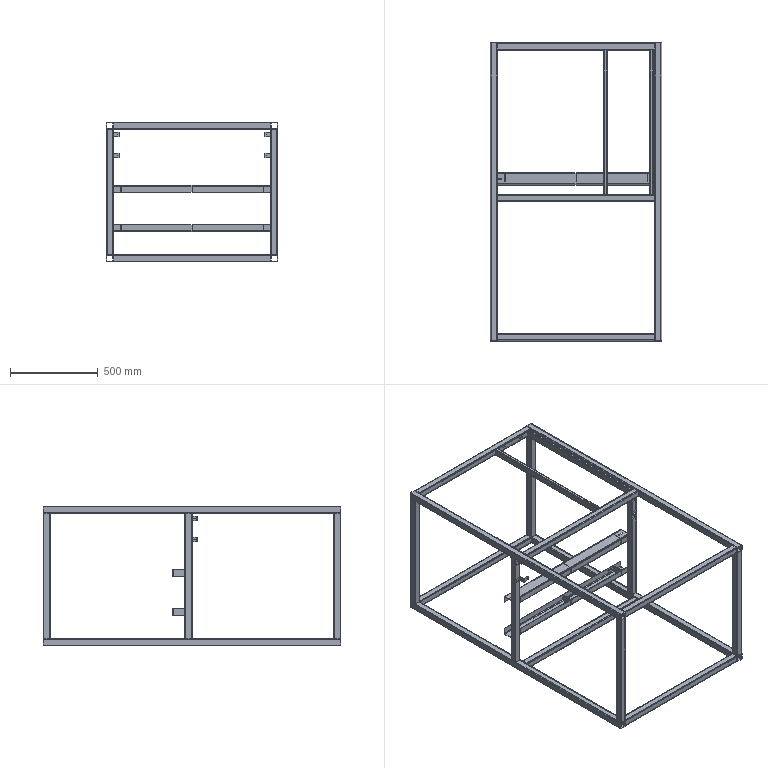Part | STEP file | Coffee machine structure frame 01001_default<by machining> | 38 solids | 656 faces | box 977 x 1697 x 797 mm | volume 7192337 mm3 | plane 396 | cylinder 260 | commonest cylinder face diameters 2.5 x78 5 x64 10 x64 6 x18 8 x16 3 x8